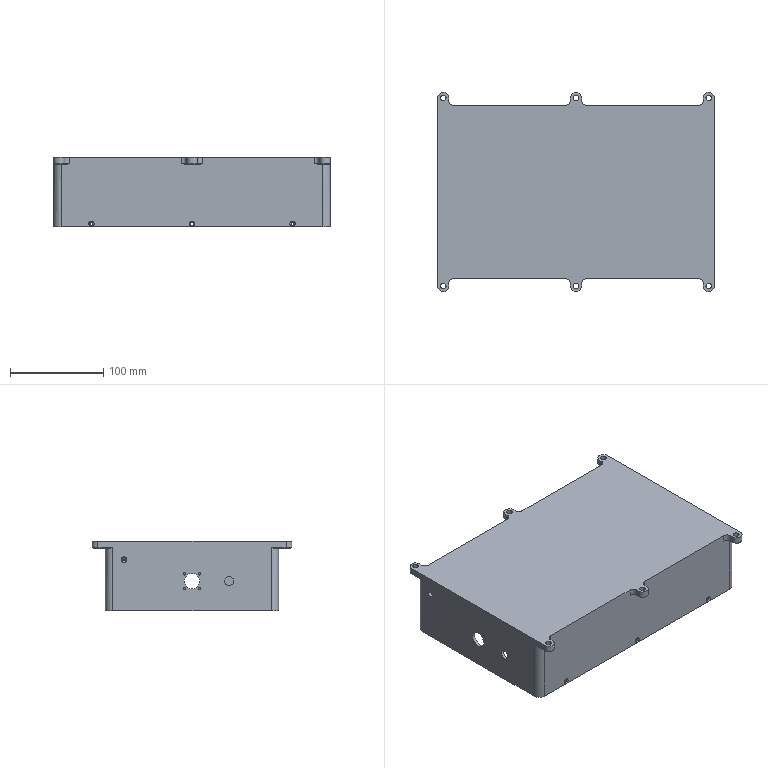NC program | NX | posted with a generic post | part box 297 x 214 x 75 mm
Whole program:
N10 G17 G21 G94 G90
(PLANAR_MILL_COPY_COPY_COPY_COPY_COPY_COPY , TOOL : D6A45)
N12 T01 M6
N14 G54
N16 G17 G0 G90 X36.649 Y-41.99 B0. C0. S9500 M3
N18 G43 Z30. H1
N20 Z0.
N22 G94 G1 Z-1. F1250.
N24 X36.4 Y-42.134
N26 G3 X35.9 Y-43. R1.
N28 X40. Y-47.1 R4.1
N30 X35.9 Y-43. R-4.1
N32 X36.4 Y-43.866 R1.
N34 G1 X36.649 Y-44.01
N36 Z0.
N38 G0 Z30.
N40 X6.681 Y-43.964
N42 Z0.
N44 G1 Z-1.
N46 X6.85 Y-43.866
N48 G3 X7.35 Y-43. R1.
N50 X0. Y-35.65 R7.35
N52 X7.35 Y-43. R-7.35
N54 X6.85 Y-42.134 R1.
N56 G1 X6.681 Y-42.036
N58 Z0.
N60 G0 Z30.
N62 X-71.654 Y-20.717
N64 Z0.
N66 G1 Z-1.
N68 X-71.375 Y-20.866
N70 G3 X-70.875 Y-20. R1.
N72 X-73. Y-17.875 R2.125
N74 X-70.875 Y-20. R-2.125
N76 X-71.375 Y-19.134 R1.
N78 G1 X-71.654 Y-19.283
N80 Z0.
N82 G0 Z30.
N84 M5
N86 M2